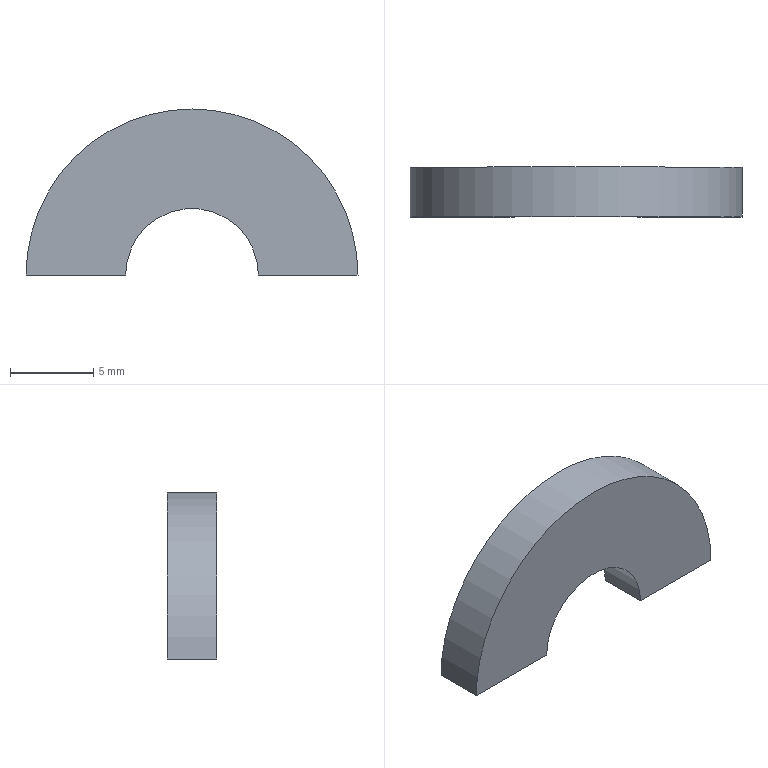Part | STEP file | Cuon T phu H01_8 | 1 solid | 6 faces | box 20 x 3 x 10 mm | volume 395.841 mm3 | plane 4 | cylinder 2 | commonest cylinder face diameters 8 x1 20 x1
STEP:
#1=CARTESIAN_POINT('',(0.,0.,0.));
#2=DIRECTION('',(0.,0.,1.));
#3=DIRECTION('',(1.,0.,0.));
#4=AXIS2_PLACEMENT_3D('',#1,#2,#3);
#5=CARTESIAN_POINT('',(-10.,3.,0.));
#6=VERTEX_POINT('',#5);
#7=CARTESIAN_POINT('',(-4.,3.,0.));
#8=VERTEX_POINT('',#7);
#9=CARTESIAN_POINT('',(0.,3.,0.));
#10=DIRECTION('',(1.,0.,0.));
#11=VECTOR('',#10,1.);
#12=LINE('',#9,#11);
#13=CARTESIAN_POINT('',(0.,3.,0.));
#14=DIRECTION('',(0.,1.,0.));
#15=DIRECTION('',(0.,0.,1.));
#16=AXIS2_PLACEMENT_3D('',#13,#14,#15);
#17=PLANE('',#16);
#18=CARTESIAN_POINT('',(0.,0.));
#19=DIRECTION('',(0.,1.));
#20=VECTOR('',#19,1.);
#21=LINE('',#18,#20);
#22=(GEOMETRIC_REPRESENTATION_CONTEXT(2)PARAMETRIC_REPRESENTATION_CONTEXT()REPRESENTATION_CONTEXT('',''));
#23=DEFINITIONAL_REPRESENTATION('',(#21),#22);
#24=PCURVE('',#17,#23);
#25=CARTESIAN_POINT('',(120.,-95.57,0.));
#26=DIRECTION('',(0.,0.,1.));
#27=DIRECTION('',(1.,0.,0.));
#28=AXIS2_PLACEMENT_3D('',#25,#26,#27);
#29=PLANE('',#28);
#30=CARTESIAN_POINT('',(-120.,98.57));
#31=DIRECTION('',(1.,0.));
#32=VECTOR('',#31,1.);
#33=LINE('',#30,#32);
#34=(GEOMETRIC_REPRESENTATION_CONTEXT(2)PARAMETRIC_REPRESENTATION_CONTEXT()REPRESENTATION_CONTEXT('',''));
#35=DEFINITIONAL_REPRESENTATION('',(#33),#34);
#36=PCURVE('',#29,#35);
#37=SURFACE_CURVE('',#12,(#24,#36),.PCURVE_S1.);
#38=EDGE_CURVE('',#6,#8,#37,.T.);
#39=ORIENTED_EDGE('',*,*,#38,.F.);
#40=CARTESIAN_POINT('',(10.,3.,0.));
#41=VERTEX_POINT('',#40);
#42=CARTESIAN_POINT('',(0.,3.,0.));
#43=DIRECTION('',(0.,1.,0.));
#44=DIRECTION('',(0.,0.,1.));
#45=AXIS2_PLACEMENT_3D('',#42,#43,#44);
#46=CIRCLE('',#45,10.);
#47=CARTESIAN_POINT('',(0.,0.));
#48=DIRECTION('',(1.,0.));
#49=AXIS2_PLACEMENT_2D('',#47,#48);
#50=CIRCLE('',#49,10.);
#51=(GEOMETRIC_REPRESENTATION_CONTEXT(2)PARAMETRIC_REPRESENTATION_CONTEXT()REPRESENTATION_CONTEXT('',''));
#52=DEFINITIONAL_REPRESENTATION('',(#50),#51);
#53=PCURVE('',#17,#52);
#54=CARTESIAN_POINT('',(0.,3.,0.));
#55=DIRECTION('',(0.,-1.,0.));
#56=DIRECTION('',(0.,0.,-1.));
#57=AXIS2_PLACEMENT_3D('',#54,#55,#56);
#58=CYLINDRICAL_SURFACE('',#57,10.);
#59=CARTESIAN_POINT('',(9.425,0.));
#60=DIRECTION('',(-1.,0.));
#61=VECTOR('',#60,1.);
#62=LINE('',#59,#61);
#63=(GEOMETRIC_REPRESENTATION_CONTEXT(2)PARAMETRIC_REPRESENTATION_CONTEXT()REPRESENTATION_CONTEXT('',''));
#64=DEFINITIONAL_REPRESENTATION('',(#62),#63);
#65=PCURVE('',#58,#64);
#66=SURFACE_CURVE('',#46,(#53,#65),.PCURVE_S1.);
#67=EDGE_CURVE('',#6,#41,#66,.T.);
#68=ORIENTED_EDGE('',*,*,#67,.T.);
#69=CARTESIAN_POINT('',(4.,3.,0.));
#70=VERTEX_POINT('',#69);
#71=CARTESIAN_POINT('',(0.,3.,0.));
#72=DIRECTION('',(1.,0.,0.));
#73=VECTOR('',#72,1.);
#74=LINE('',#71,#73);
#75=CARTESIAN_POINT('',(0.,0.));
#76=DIRECTION('',(0.,1.));
#77=VECTOR('',#76,1.);
#78=LINE('',#75,#77);
#79=(GEOMETRIC_REPRESENTATION_CONTEXT(2)PARAMETRIC_REPRESENTATION_CONTEXT()REPRESENTATION_CONTEXT('',''));
#80=DEFINITIONAL_REPRESENTATION('',(#78),#79);
#81=PCURVE('',#17,#80);
#82=CARTESIAN_POINT('',(120.,-95.57,0.));
#83=DIRECTION('',(0.,0.,1.));
#84=DIRECTION('',(1.,0.,0.));
#85=AXIS2_PLACEMENT_3D('',#82,#83,#84);
#86=PLANE('',#85);
#87=CARTESIAN_POINT('',(-120.,98.57));
#88=DIRECTION('',(1.,0.));
#89=VECTOR('',#88,1.);
#90=LINE('',#87,#89);
#91=(GEOMETRIC_REPRESENTATION_CONTEXT(2)PARAMETRIC_REPRESENTATION_CONTEXT()REPRESENTATION_CONTEXT('',''));
#92=DEFINITIONAL_REPRESENTATION('',(#90),#91);
#93=PCURVE('',#86,#92);
#94=SURFACE_CURVE('',#74,(#81,#93),.PCURVE_S1.);
#95=EDGE_CURVE('',#70,#41,#94,.T.);
#96=ORIENTED_EDGE('',*,*,#95,.F.);
#97=CARTESIAN_POINT('',(0.,3.,0.));
#98=DIRECTION('',(0.,1.,0.));
#99=DIRECTION('',(0.,0.,1.));
#100=AXIS2_PLACEMENT_3D('',#97,#98,#99);
#101=CIRCLE('',#100,4.);
#102=CARTESIAN_POINT('',(0.,0.));
#103=DIRECTION('',(1.,0.));
#104=AXIS2_PLACEMENT_2D('',#102,#103);
#105=CIRCLE('',#104,4.);
#106=(GEOMETRIC_REPRESENTATION_CONTEXT(2)PARAMETRIC_REPRESENTATION_CONTEXT()REPRESENTATION_CONTEXT('',''));
#107=DEFINITIONAL_REPRESENTATION('',(#105),#106);
#108=PCURVE('',#17,#107);
#109=CARTESIAN_POINT('',(0.,3.,0.));
#110=DIRECTION('',(0.,-1.,0.));
#111=DIRECTION('',(0.,0.,-1.));
#112=AXIS2_PLACEMENT_3D('',#109,#110,#111);
#113=CYLINDRICAL_SURFACE('',#112,4.);
#114=CARTESIAN_POINT('',(9.425,0.));
#115=DIRECTION('',(-1.,0.));
#116=VECTOR('',#115,1.);
#117=LINE('',#114,#116);
#118=(GEOMETRIC_REPRESENTATION_CONTEXT(2)PARAMETRIC_REPRESENTATION_CONTEXT()REPRESENTATION_CONTEXT('',''));
#119=DEFINITIONAL_REPRESENTATION('',(#117),#118);
#120=PCURVE('',#113,#119);
#121=SURFACE_CURVE('',#101,(#108,#120),.PCURVE_S1.);
#122=EDGE_CURVE('',#8,#70,#121,.T.);
#123=ORIENTED_EDGE('',*,*,#122,.F.);
#124=EDGE_LOOP('',(#39,#68,#96,#123));
#125=FACE_BOUND('',#124,.T.);
#126=ADVANCED_FACE('',(#125),#17,.T.);
#127=CARTESIAN_POINT('',(-10.,0.,0.));
#128=VERTEX_POINT('',#127);
#129=CARTESIAN_POINT('',(10.,0.,0.));
#130=VERTEX_POINT('',#129);
#131=CARTESIAN_POINT('',(0.,0.,0.));
#132=DIRECTION('',(0.,1.,0.));
#133=DIRECTION('',(0.,0.,1.));
#134=AXIS2_PLACEMENT_3D('',#131,#132,#133);
#135=CIRCLE('',#134,10.);
#136=CARTESIAN_POINT('',(0.,0.,0.));
#137=DIRECTION('',(0.,1.,0.));
#138=DIRECTION('',(0.,0.,1.));
#139=AXIS2_PLACEMENT_3D('',#136,#137,#138);
#140=PLANE('',#139);
#141=CARTESIAN_POINT('',(0.,0.));
#142=DIRECTION('',(1.,0.));
#143=AXIS2_PLACEMENT_2D('',#141,#142);
#144=CIRCLE('',#143,10.);
#145=(GEOMETRIC_REPRESENTATION_CONTEXT(2)PARAMETRIC_REPRESENTATION_CONTEXT()REPRESENTATION_CONTEXT('',''));
#146=DEFINITIONAL_REPRESENTATION('',(#144),#145);
#147=PCURVE('',#140,#146);
#148=CARTESIAN_POINT('',(9.425,3.));
#149=DIRECTION('',(-1.,0.));
#150=VECTOR('',#149,1.);
#151=LINE('',#148,#150);
#152=(GEOMETRIC_REPRESENTATION_CONTEXT(2)PARAMETRIC_REPRESENTATION_CONTEXT()REPRESENTATION_CONTEXT('',''));
#153=DEFINITIONAL_REPRESENTATION('',(#151),#152);
#154=PCURVE('',#58,#153);
#155=SURFACE_CURVE('',#135,(#147,#154),.PCURVE_S1.);
#156=EDGE_CURVE('',#128,#130,#155,.T.);
#157=ORIENTED_EDGE('',*,*,#156,.F.);
#158=CARTESIAN_POINT('',(-4.,0.,0.));
#159=VERTEX_POINT('',#158);
#160=CARTESIAN_POINT('',(0.,0.,0.));
#161=DIRECTION('',(1.,0.,0.));
#162=VECTOR('',#161,1.);
#163=LINE('',#160,#162);
#164=CARTESIAN_POINT('',(0.,0.));
#165=DIRECTION('',(0.,1.));
#166=VECTOR('',#165,1.);
#167=LINE('',#164,#166);
#168=(GEOMETRIC_REPRESENTATION_CONTEXT(2)PARAMETRIC_REPRESENTATION_CONTEXT()REPRESENTATION_CONTEXT('',''));
#169=DEFINITIONAL_REPRESENTATION('',(#167),#168);
#170=PCURVE('',#140,#169);
#171=CARTESIAN_POINT('',(-120.,95.57));
#172=DIRECTION('',(1.,0.));
#173=VECTOR('',#172,1.);
#174=LINE('',#171,#173);
#175=(GEOMETRIC_REPRESENTATION_CONTEXT(2)PARAMETRIC_REPRESENTATION_CONTEXT()REPRESENTATION_CONTEXT('',''));
#176=DEFINITIONAL_REPRESENTATION('',(#174),#175);
#177=PCURVE('',#29,#176);
#178=SURFACE_CURVE('',#163,(#170,#177),.PCURVE_S1.);
#179=EDGE_CURVE('',#128,#159,#178,.T.);
#180=ORIENTED_EDGE('',*,*,#179,.T.);
#181=CARTESIAN_POINT('',(4.,0.,0.));
#182=VERTEX_POINT('',#181);
#183=CARTESIAN_POINT('',(0.,0.,0.));
#184=DIRECTION('',(0.,1.,0.));
#185=DIRECTION('',(0.,0.,1.));
#186=AXIS2_PLACEMENT_3D('',#183,#184,#185);
#187=CIRCLE('',#186,4.);
#188=CARTESIAN_POINT('',(0.,0.));
#189=DIRECTION('',(1.,0.));
#190=AXIS2_PLACEMENT_2D('',#188,#189);
#191=CIRCLE('',#190,4.);
#192=(GEOMETRIC_REPRESENTATION_CONTEXT(2)PARAMETRIC_REPRESENTATION_CONTEXT()REPRESENTATION_CONTEXT('',''));
#193=DEFINITIONAL_REPRESENTATION('',(#191),#192);
#194=PCURVE('',#140,#193);
#195=CARTESIAN_POINT('',(9.425,3.));
#196=DIRECTION('',(-1.,0.));
#197=VECTOR('',#196,1.);
#198=LINE('',#195,#197);
#199=(GEOMETRIC_REPRESENTATION_CONTEXT(2)PARAMETRIC_REPRESENTATION_CONTEXT()REPRESENTATION_CONTEXT('',''));
#200=DEFINITIONAL_REPRESENTATION('',(#198),#199);
#201=PCURVE('',#113,#200);
#202=SURFACE_CURVE('',#187,(#194,#201),.PCURVE_S1.);
#203=EDGE_CURVE('',#159,#182,#202,.T.);
#204=ORIENTED_EDGE('',*,*,#203,.T.);
#205=CARTESIAN_POINT('',(0.,0.,0.));
#206=DIRECTION('',(1.,0.,0.));
#207=VECTOR('',#206,1.);
#208=LINE('',#205,#207);
#209=CARTESIAN_POINT('',(0.,0.));
#210=DIRECTION('',(0.,1.));
#211=VECTOR('',#210,1.);
#212=LINE('',#209,#211);
#213=(GEOMETRIC_REPRESENTATION_CONTEXT(2)PARAMETRIC_REPRESENTATION_CONTEXT()REPRESENTATION_CONTEXT('',''));
#214=DEFINITIONAL_REPRESENTATION('',(#212),#213);
#215=PCURVE('',#140,#214);
#216=CARTESIAN_POINT('',(-120.,95.57));
#217=DIRECTION('',(1.,0.));
#218=VECTOR('',#217,1.);
#219=LINE('',#216,#218);
#220=(GEOMETRIC_REPRESENTATION_CONTEXT(2)PARAMETRIC_REPRESENTATION_CONTEXT()REPRESENTATION_CONTEXT('',''));
#221=DEFINITIONAL_REPRESENTATION('',(#219),#220);
#222=PCURVE('',#86,#221);
#223=SURFACE_CURVE('',#208,(#215,#222),.PCURVE_S1.);
#224=EDGE_CURVE('',#182,#130,#223,.T.);
#225=ORIENTED_EDGE('',*,*,#224,.T.);
#226=EDGE_LOOP('',(#157,#180,#204,#225));
#227=FACE_BOUND('',#226,.T.);
#228=ADVANCED_FACE('',(#227),#140,.F.);
#229=ORIENTED_EDGE('',*,*,#67,.F.);
#230=CARTESIAN_POINT('',(-10.,3.,0.));
#231=DIRECTION('',(0.,-1.,0.));
#232=VECTOR('',#231,1.);
#233=LINE('',#230,#232);
#234=CARTESIAN_POINT('',(4.712,0.));
#235=DIRECTION('',(0.,1.));
#236=VECTOR('',#235,1.);
#237=LINE('',#234,#236);
#238=(GEOMETRIC_REPRESENTATION_CONTEXT(2)PARAMETRIC_REPRESENTATION_CONTEXT()REPRESENTATION_CONTEXT('',''));
#239=DEFINITIONAL_REPRESENTATION('',(#237),#238);
#240=PCURVE('',#58,#239);
#241=CARTESIAN_POINT('',(-130.,98.57));
#242=DIRECTION('',(0.,-1.));
#243=VECTOR('',#242,1.);
#244=LINE('',#241,#243);
#245=(GEOMETRIC_REPRESENTATION_CONTEXT(2)PARAMETRIC_REPRESENTATION_CONTEXT()REPRESENTATION_CONTEXT('',''));
#246=DEFINITIONAL_REPRESENTATION('',(#244),#245);
#247=PCURVE('',#29,#246);
#248=SURFACE_CURVE('',#233,(#240,#247),.PCURVE_S1.);
#249=EDGE_CURVE('',#6,#128,#248,.T.);
#250=ORIENTED_EDGE('',*,*,#249,.T.);
#251=ORIENTED_EDGE('',*,*,#156,.T.);
#252=CARTESIAN_POINT('',(10.,3.,0.));
#253=DIRECTION('',(0.,1.,0.));
#254=VECTOR('',#253,1.);
#255=LINE('',#252,#254);
#256=CARTESIAN_POINT('',(1.571,0.));
#257=DIRECTION('',(0.,-1.));
#258=VECTOR('',#257,1.);
#259=LINE('',#256,#258);
#260=(GEOMETRIC_REPRESENTATION_CONTEXT(2)PARAMETRIC_REPRESENTATION_CONTEXT()REPRESENTATION_CONTEXT('',''));
#261=DEFINITIONAL_REPRESENTATION('',(#259),#260);
#262=PCURVE('',#58,#261);
#263=CARTESIAN_POINT('',(-110.,98.57));
#264=DIRECTION('',(0.,1.));
#265=VECTOR('',#264,1.);
#266=LINE('',#263,#265);
#267=(GEOMETRIC_REPRESENTATION_CONTEXT(2)PARAMETRIC_REPRESENTATION_CONTEXT()REPRESENTATION_CONTEXT('',''));
#268=DEFINITIONAL_REPRESENTATION('',(#266),#267);
#269=PCURVE('',#86,#268);
#270=SURFACE_CURVE('',#255,(#262,#269),.PCURVE_S1.);
#271=EDGE_CURVE('',#130,#41,#270,.T.);
#272=ORIENTED_EDGE('',*,*,#271,.T.);
#273=EDGE_LOOP('',(#229,#250,#251,#272));
#274=FACE_BOUND('',#273,.T.);
#275=ADVANCED_FACE('',(#274),#58,.T.);
#276=ORIENTED_EDGE('',*,*,#203,.T.);
#277=CARTESIAN_POINT('',(4.,3.,0.));
#278=DIRECTION('',(0.,1.,0.));
#279=VECTOR('',#278,1.);
#280=LINE('',#277,#279);
#281=CARTESIAN_POINT('',(1.571,0.));
#282=DIRECTION('',(0.,-1.));
#283=VECTOR('',#282,1.);
#284=LINE('',#281,#283);
#285=(GEOMETRIC_REPRESENTATION_CONTEXT(2)PARAMETRIC_REPRESENTATION_CONTEXT()REPRESENTATION_CONTEXT('',''));
#286=DEFINITIONAL_REPRESENTATION('',(#284),#285);
#287=PCURVE('',#113,#286);
#288=CARTESIAN_POINT('',(-116.,98.57));
#289=DIRECTION('',(0.,1.));
#290=VECTOR('',#289,1.);
#291=LINE('',#288,#290);
#292=(GEOMETRIC_REPRESENTATION_CONTEXT(2)PARAMETRIC_REPRESENTATION_CONTEXT()REPRESENTATION_CONTEXT('',''));
#293=DEFINITIONAL_REPRESENTATION('',(#291),#292);
#294=PCURVE('',#86,#293);
#295=SURFACE_CURVE('',#280,(#287,#294),.PCURVE_S1.);
#296=EDGE_CURVE('',#182,#70,#295,.T.);
#297=ORIENTED_EDGE('',*,*,#296,.T.);
#298=ORIENTED_EDGE('',*,*,#122,.F.);
#299=CARTESIAN_POINT('',(-4.,3.,0.));
#300=DIRECTION('',(0.,-1.,0.));
#301=VECTOR('',#300,1.);
#302=LINE('',#299,#301);
#303=CARTESIAN_POINT('',(4.712,0.));
#304=DIRECTION('',(0.,1.));
#305=VECTOR('',#304,1.);
#306=LINE('',#303,#305);
#307=(GEOMETRIC_REPRESENTATION_CONTEXT(2)PARAMETRIC_REPRESENTATION_CONTEXT()REPRESENTATION_CONTEXT('',''));
#308=DEFINITIONAL_REPRESENTATION('',(#306),#307);
#309=PCURVE('',#113,#308);
#310=CARTESIAN_POINT('',(-124.,98.57));
#311=DIRECTION('',(0.,-1.));
#312=VECTOR('',#311,1.);
#313=LINE('',#310,#312);
#314=(GEOMETRIC_REPRESENTATION_CONTEXT(2)PARAMETRIC_REPRESENTATION_CONTEXT()REPRESENTATION_CONTEXT('',''));
#315=DEFINITIONAL_REPRESENTATION('',(#313),#314);
#316=PCURVE('',#29,#315);
#317=SURFACE_CURVE('',#302,(#309,#316),.PCURVE_S1.);
#318=EDGE_CURVE('',#8,#159,#317,.T.);
#319=ORIENTED_EDGE('',*,*,#318,.T.);
#320=EDGE_LOOP('',(#276,#297,#298,#319));
#321=FACE_BOUND('',#320,.F.);
#322=ADVANCED_FACE('',(#321),#113,.F.);
#323=ORIENTED_EDGE('',*,*,#224,.F.);
#324=ORIENTED_EDGE('',*,*,#296,.T.);
#325=ORIENTED_EDGE('',*,*,#95,.T.);
#326=ORIENTED_EDGE('',*,*,#271,.F.);
#327=EDGE_LOOP('',(#323,#324,#325,#326));
#328=FACE_BOUND('',#327,.T.);
#329=ADVANCED_FACE('',(#328),#86,.F.);
#330=ORIENTED_EDGE('',*,*,#38,.T.);
#331=ORIENTED_EDGE('',*,*,#318,.T.);
#332=ORIENTED_EDGE('',*,*,#179,.F.);
#333=ORIENTED_EDGE('',*,*,#249,.F.);
#334=EDGE_LOOP('',(#330,#331,#332,#333));
#335=FACE_BOUND('',#334,.T.);
#336=ADVANCED_FACE('',(#335),#29,.F.);
#337=CLOSED_SHELL('',(#126,#228,#275,#322,#329,#336));
#338=MANIFOLD_SOLID_BREP('',#337);
#339=(LENGTH_UNIT()NAMED_UNIT(*)SI_UNIT(.MILLI.,.METRE.));
#340=UNCERTAINTY_MEASURE_WITH_UNIT(LENGTH_MEASURE(0.0000001),#339,'','');
#341=(NAMED_UNIT(*)PLANE_ANGLE_UNIT()SI_UNIT($,.RADIAN.));
#342=(NAMED_UNIT(*)SI_UNIT($,.STERADIAN.)SOLID_ANGLE_UNIT());
#343=(GEOMETRIC_REPRESENTATION_CONTEXT(3)GLOBAL_UNCERTAINTY_ASSIGNED_CONTEXT((#340))GLOBAL_UNIT_ASSIGNED_CONTEXT((#339,#341,#342))REPRESENTATION_CONTEXT('',''));
#344=ADVANCED_BREP_SHAPE_REPRESENTATION('',(#4,#338),#343);